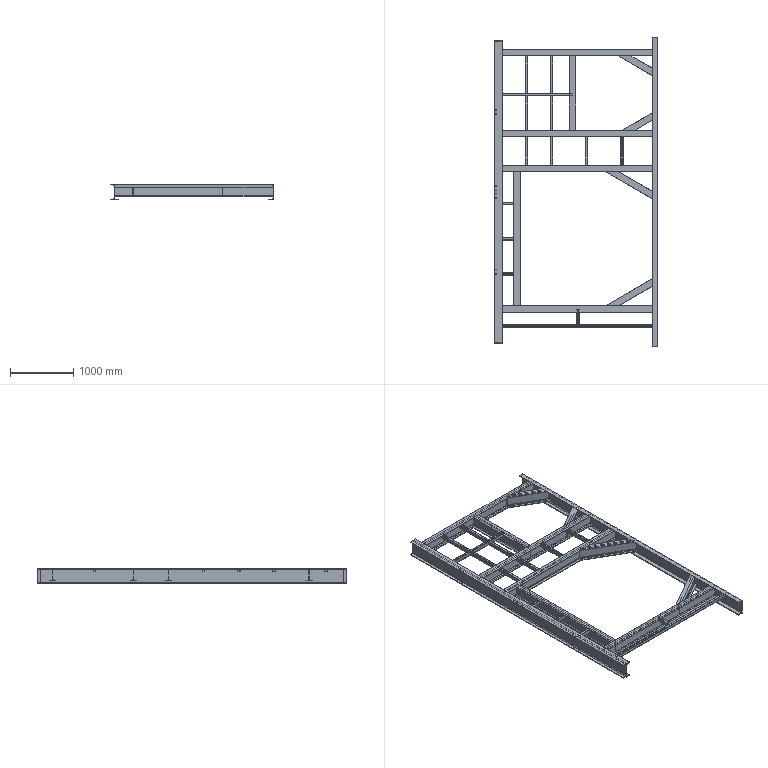Part | STEP file | PN_0020 third-floor right platform 1_Default<As Machined> | 26 solids | 675 faces | box 2578 x 4889 x 250 mm | volume 86538264 mm3 | plane 475 | cylinder 200 | commonest cylinder face diameters 26 x68 12 x58 6 x56 6.8 x8 18 x8 24 x2